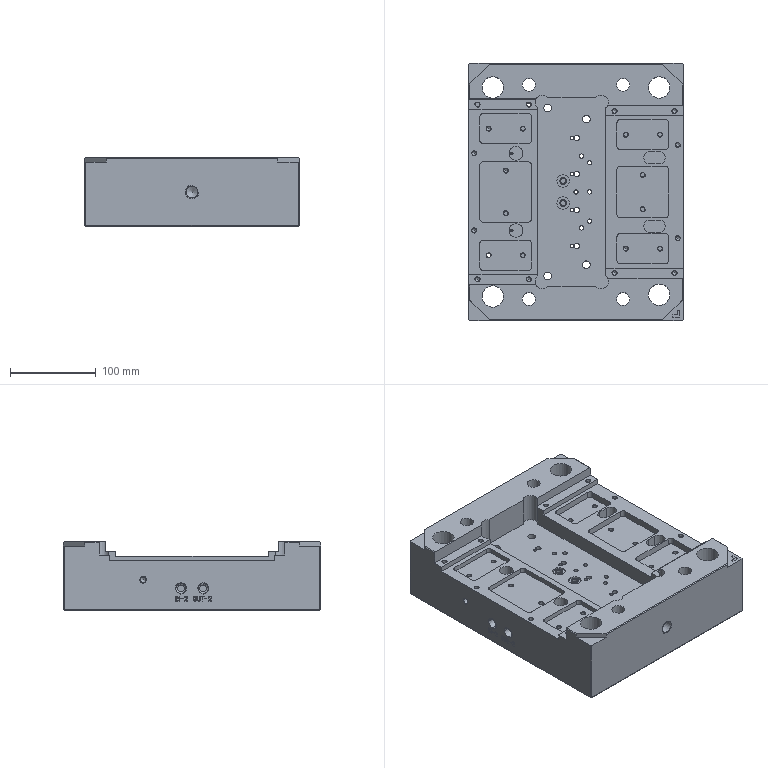NC program | PowerMill | posted with a generic post | part box 250 x 300 x 80 mm
Whole program:
%
O0001
N104 ( POWERMILL CB  : 2026004.0)
N105 ( POST VER      : 2026.0.0.5161)
N106 ( OPTION FILE   : FANUC)
N107 ( OUTPUT WORKPLANE : 1)
N108 (  )
N109 ( TOOL LIST )
N110 (-----------------------------------)
N111 ( NO. | ID    | DIA.| TIP RAD|LENGTH)
N112 (-----------------------------------)
N113 (    1|￠5_1_1| 5.0 |  0.0   |139.6 )
N114 (-----------------------------------)
N115 (  )
N116 ( NUMBER OF TOOLPATHS: 1.0 )
N117 ( ESTIMATED PROGRAM DURATION: 0 HOURS 5 MIN 54 SEC)
N118 (  )
N119 G00 G21 G80 G40 G17
N120 G90
N121 G54
N122 G53 Z0.0
N123 (---------------)
N124 ( START TOOLPATH : 30开粗-￠5-钻孔加工 )
N125 (---------------)
N126 ( TOOL NO.    :1 )
N127 ( TOOL TYPE   : DRILL)
N128 ( TOOL ID     : ￠5_1_1)
N129 ( TOOL DIA    : 5.0 LENGTH 139.6)
N130 T1
N131 M6
N132 S700 M03
N133 G00 G90 X-34.0 Y-16.0
N134 G43 Z20.0 H1
N135
N136 G05 P10000 R8
N137 Z11.0
N138 G01 Z-2.0 F80.0
N139 G00 Z11.0
N140 Z-1.4
N141 G01 Z-5.0
N142 G00 Z11.0
N143 Z-4.4
N144 G01 Z-8.0
N145 G00 Z11.0
N146 Z-7.4
N147 G01 Z-11.0
N148 G00 Z11.0
N149 Z-10.4
N150 G01 Z-14.0
N151 G00 Z11.0
N152 Z-13.4
N153 G01 Z-17.0
N154 G00 Z11.0
N155 Z-16.4
N156 G01 Z-20.0
N157 G00 Z11.0
N158 Z-19.4
N159 G01 Z-23.0
N160 G00 Z11.0
N161 Z-22.4
N162 G01 Z-26.0
N163 G00 Z11.0
N164 Z-25.4
N165 G01 Z-29.0
N166 G00 Z11.0
N167 Z-28.4
N168 G01 Z-32.0
N169 G00 Z11.0
N170 Z-31.4
N171 G01 Z-35.0
N172 G00 Z11.0
N173 Z-34.4
N174 G01 Z-38.0
N175 G00 Z11.0
N176 Z-37.4
N177 G01 Z-41.0
N178 G00 Z11.0
N179 Z-40.4
N180 G01 Z-44.0
N181 G00 Z11.0
N182 Z-43.4
N183 G01 Z-47.0
N184 G00 Z11.0
N185 Z-46.4
N186 G01 Z-48.3413
N187 G00 Z20.0
N188 X-42.0 Y-6.5
N189 Z11.0
N190 G01 Z-2.0
N191 G00 Z11.0
N192 Z-1.4
N193 G01 Z-5.0
N194 G00 Z11.0
N195 Z-4.4
N196 G01 Z-8.0
N197 G00 Z11.0
N198 Z-7.4
N199 G01 Z-11.0
N200 G00 Z11.0
N201 Z-10.4
N202 G01 Z-14.0
N203 G00 Z11.0
N204 Z-13.4
N205 G01 Z-17.0
N206 G00 Z11.0
N207 Z-16.4
N208 G01 Z-20.0
N209 G00 Z11.0
N210 Z-19.4
N211 G01 Z-23.0
N212 G00 Z11.0
N213 Z-22.4
N214 G01 Z-26.0
N215 G00 Z11.0
N216 Z-25.4
N217 G01 Z-29.0
N218 G00 Z11.0
N219 Z-28.4
N220 G01 Z-32.0
N221 G00 Z11.0
N222 Z-31.4
N223 G01 Z-35.0
N224 G00 Z11.0
N225 Z-34.4
N226 G01 Z-38.0
N227 G00 Z11.0
N228 Z-37.4
N229 G01 Z-41.0
N230 G00 Z11.0
N231 Z-40.4
N232 G01 Z-44.0
N233 G00 Z11.0
N234 Z-43.4
N235 G01 Z-47.0
N236 G00 Z11.0
N237 Z-46.4
N238 G01 Z-48.3413
N239 G00 Z20.0
N240 X0.0 Y0.0
N241 Z11.0
N242 G01 Z-2.0
N243 G00 Z11.0
N244 Z-1.4
N245 G01 Z-5.0
N246 G00 Z11.0
N247 Z-4.4
N248 G01 Z-8.0
N249 G00 Z11.0
N250 Z-7.4
N251 G01 Z-11.0
N252 G00 Z11.0
N253 Z-10.4
N254 G01 Z-14.0
N255 G00 Z11.0
N256 Z-13.4
N257 G01 Z-17.0
N258 G00 Z11.0
N259 Z-16.4
N260 G01 Z-20.0
N261 G00 Z11.0
N262 Z-19.4
N263 G01 Z-23.0
N264 G00 Z11.0
N265 Z-22.4
N266 G01 Z-26.0
N267 G00 Z11.0
N268 Z-25.4
N269 G01 Z-29.0
N270 G00 Z11.0
N271 Z-28.4
N272 G01 Z-32.0
N273 G00 Z11.0
N274 Z-31.4
N275 G01 Z-35.0
N276 G00 Z11.0
N277 Z-34.4
N278 G01 Z-38.0
N279 G00 Z11.0
N280 Z-37.4
N281 G01 Z-41.0
N282 G00 Z11.0
N283 Z-40.4
N284 G01 Z-44.0
N285 G00 Z11.0
N286 Z-43.4
N287 G01 Z-47.0
N288 G00 Z11.0
N289 Z-46.4
N290 G01 Z-48.3413
N291 G00 Z20.0
N292 Y-16.0
N293 Z11.0
N294 G01 Z-2.0
N295 G00 Z11.0
N296 Z-1.4
N297 G01 Z-5.0
N298 G00 Z11.0
N299 Z-4.4
N300 G01 Z-8.0
N301 G00 Z11.0
N302 Z-7.4
N303 G01 Z-11.0
N304 G00 Z11.0
N305 Z-10.4
N306 G01 Z-14.0
N307 G00 Z11.0
N308 Z-13.4
N309 G01 Z-17.0
N310 G00 Z11.0
N311 Z-16.4
N312 G01 Z-20.0
N313 G00 Z11.0
N314 Z-19.4
N315 G01 Z-23.0
N316 G00 Z11.0
N317 Z-22.4
N318 G01 Z-26.0
N319 G00 Z11.0
N320 Z-25.4
N321 G01 Z-29.0
N322 G00 Z11.0
N323 Z-28.4
N324 G01 Z-32.0
N325 G00 Z11.0
N326 Z-31.4
N327 G01 Z-35.0
N328 G00 Z11.0
N329 Z-34.4
N330 G01 Z-38.0
N331 G00 Z11.0
N332 Z-37.4
N333 G01 Z-41.0
N334 G00 Z11.0
N335 Z-40.4
N336 G01 Z-44.0
N337 G00 Z11.0
N338 Z-43.4
N339 G01 Z-47.0
N340 G00 Z11.0
N341 Z-46.4
N342 G01 Z-48.3413
N343 G00 Z20.0
N344 X34.0
N345 Z11.0
N346 G01 Z-2.0
N347 G00 Z11.0
N348 Z-1.4
N349 G01 Z-5.0
N350 G00 Z11.0
N351 Z-4.4
N352 G01 Z-8.0
N353 G00 Z11.0
N354 Z-7.4
N355 G01 Z-11.0
N356 G00 Z11.0
N357 Z-10.4
N358 G01 Z-14.0
N359 G00 Z11.0
N360 Z-13.4
N361 G01 Z-17.0
N362 G00 Z11.0
N363 Z-16.4
N364 G01 Z-20.0
N365 G00 Z11.0
N366 Z-19.4
N367 G01 Z-23.0
N368 G00 Z11.0
N369 Z-22.4
N370 G01 Z-26.0
N371 G00 Z11.0
N372 Z-25.4
N373 G01 Z-29.0
N374 G00 Z11.0
N375 Z-28.4
N376 G01 Z-32.0
N377 G00 Z11.0
N378 Z-31.4
N379 G01 Z-35.0
N380 G00 Z11.0
N381 Z-34.4
N382 G01 Z-38.0
N383 G00 Z11.0
N384 Z-37.4
N385 G01 Z-41.0
N386 G00 Z11.0
N387 Z-40.4
N388 G01 Z-44.0
N389 G00 Z11.0
N390 Z-43.4
N391 G01 Z-47.0
N392 G00 Z11.0
N393 Z-46.4
N394 G01 Z-48.3413
N395 G00 Z20.0
N396 X42.0 Y-6.5
N397 Z11.0
N398 G01 Z-2.0
N399 G00 Z11.0
N400 Z-1.4
N401 G01 Z-5.0
N402 G00 Z11.0
N403 Z-4.4
N404 G01 Z-8.0
N405 G00 Z11.0
N406 Z-7.4
N407 G01 Z-11.0
N408 G00 Z11.0
N409 Z-10.4
N410 G01 Z-14.0
N411 G00 Z11.0
N412 Z-13.4
N413 G01 Z-17.0
N414 G00 Z11.0
N415 Z-16.4
N416 G01 Z-20.0
N417 G00 Z11.0
N418 Z-19.4
N419 G01 Z-23.0
N420 G00 Z11.0
N421 Z-22.4
N422 G01 Z-26.0
N423 G00 Z11.0
N424 Z-25.4
N425 G01 Z-29.0
N426 G00 Z11.0
N427 Z-28.4
N428 G01 Z-32.0
N429 G00 Z11.0
N430 Z-31.4
N431 G01 Z-35.0
N432 G00 Z11.0
N433 Z-34.4
N434 G01 Z-38.0
N435 G00 Z11.0
N436 Z-37.4
N437 G01 Z-41.0
N438 G00 Z11.0
N439 Z-40.4
N440 G01 Z-44.0
N441 G00 Z11.0
N442 Z-43.4
N443 G01 Z-47.0
N444 G00 Z11.0
N445 Z-46.4
N446 G01 Z-48.3413
N447 G00 Z20.0
N448 G05 P0
N449 (---------------)
N450 ( END TOOLPATH : 30开粗-￠5-钻孔加工 )
N451 (---------------)
N452
N453 M05
N454 G53 Z0.0
N455 M30
%